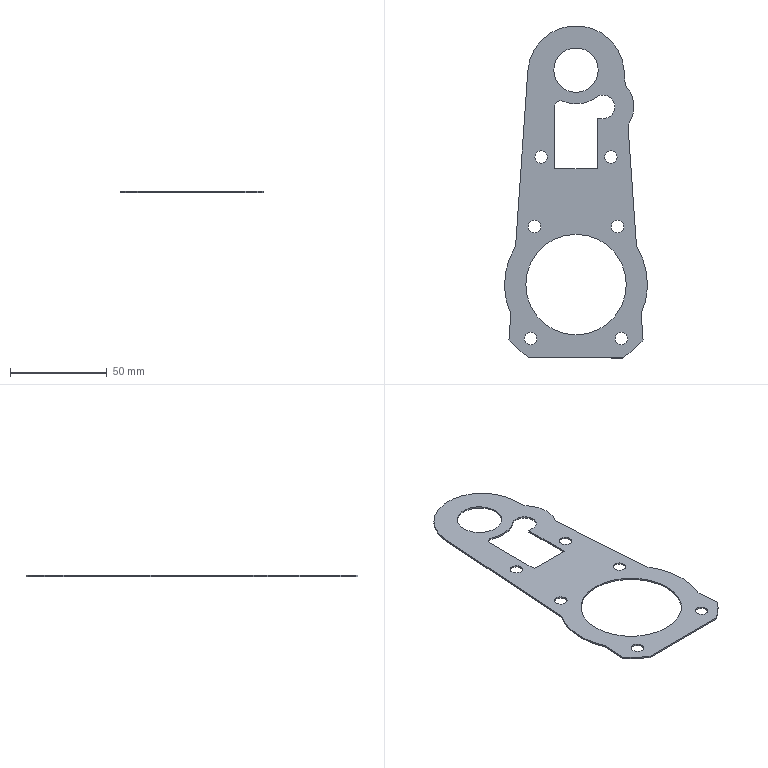Part | SolidWorks | features BaseBody 1 | 1 solid | 39 faces | box 74 x 172 x 0.8 mm | volume 5148 mm3 | cylinder 27 | plane 12 | commonest cylinder face diameters 6.5 x12 74 x3 12.2 x2 23 x2 52 x2 90 x2
STEP:
#1=CARTESIAN_POINT('',(-81.463,-50.104,-130.75));
#2=VERTEX_POINT('',#1);
#3=CARTESIAN_POINT('',(-78.207,-65.28,-130.75));
#4=VERTEX_POINT('',#3);
#5=CARTESIAN_POINT('',(-44.463,-50.104,-130.75));
#6=DIRECTION('',(0.,0.,1.));
#7=DIRECTION('',(1.,0.,0.));
#8=AXIS2_PLACEMENT_3D('',#5,#6,#7);
#9=CIRCLE('',#8,37.);
#10=EDGE_CURVE('',#2,#4,#9,.T.);
#11=ORIENTED_EDGE('',*,*,#10,.F.);
#12=CARTESIAN_POINT('',(-81.463,-50.104,-131.55));
#13=VERTEX_POINT('',#12);
#14=CARTESIAN_POINT('',(-81.463,-50.104,-130.75));
#15=DIRECTION('',(0.,0.,-1.));
#16=VECTOR('',#15,1000.);
#17=LINE('',#14,#16);
#18=EDGE_CURVE('',#2,#13,#17,.T.);
#19=ORIENTED_EDGE('',*,*,#18,.T.);
#20=CARTESIAN_POINT('',(-78.207,-65.28,-131.55));
#21=VERTEX_POINT('',#20);
#22=CARTESIAN_POINT('',(-44.463,-50.104,-131.55));
#23=DIRECTION('',(0.,0.,1.));
#24=DIRECTION('',(1.,0.,0.));
#25=AXIS2_PLACEMENT_3D('',#22,#23,#24);
#26=CIRCLE('',#25,37.);
#27=EDGE_CURVE('',#13,#21,#26,.T.);
#28=ORIENTED_EDGE('',*,*,#27,.T.);
#29=CARTESIAN_POINT('',(-78.207,-65.28,-130.75));
#30=DIRECTION('',(0.,0.,-1.));
#31=VECTOR('',#30,1000.);
#32=LINE('',#29,#31);
#33=EDGE_CURVE('',#4,#21,#32,.T.);
#34=ORIENTED_EDGE('',*,*,#33,.F.);
#35=EDGE_LOOP('',(#11,#19,#28,#34));
#36=FACE_OUTER_BOUND('',#35,.T.);
#37=CARTESIAN_POINT('',(-44.463,-50.104,-130.75));
#38=DIRECTION('',(0.,0.,-1.));
#39=DIRECTION('',(-1.,0.,0.));
#40=AXIS2_PLACEMENT_3D('',#37,#38,#39);
#41=CYLINDRICAL_SURFACE('',#40,37.);
#42=ADVANCED_FACE('',(#36),#41,.T.);
#43=CARTESIAN_POINT('',(-70.463,-50.104,-131.55));
#44=VERTEX_POINT('',#43);
#45=CARTESIAN_POINT('',(-18.463,-50.104,-131.55));
#46=VERTEX_POINT('',#45);
#47=CARTESIAN_POINT('',(-44.463,-50.104,-131.55));
#48=DIRECTION('',(0.,0.,1.));
#49=DIRECTION('',(1.,0.,0.));
#50=AXIS2_PLACEMENT_3D('',#47,#48,#49);
#51=CIRCLE('',#50,26.);
#52=EDGE_CURVE('',#44,#46,#51,.T.);
#53=ORIENTED_EDGE('',*,*,#52,.F.);
#54=CARTESIAN_POINT('',(-70.463,-50.104,-130.75));
#55=VERTEX_POINT('',#54);
#56=CARTESIAN_POINT('',(-70.463,-50.104,-131.55));
#57=DIRECTION('',(0.,0.,1.));
#58=VECTOR('',#57,1000.);
#59=LINE('',#56,#58);
#60=EDGE_CURVE('',#44,#55,#59,.T.);
#61=ORIENTED_EDGE('',*,*,#60,.T.);
#62=CARTESIAN_POINT('',(-18.463,-50.104,-130.75));
#63=VERTEX_POINT('',#62);
#64=CARTESIAN_POINT('',(-44.463,-50.104,-130.75));
#65=DIRECTION('',(0.,0.,1.));
#66=DIRECTION('',(1.,0.,0.));
#67=AXIS2_PLACEMENT_3D('',#64,#65,#66);
#68=CIRCLE('',#67,26.);
#69=EDGE_CURVE('',#55,#63,#68,.T.);
#70=ORIENTED_EDGE('',*,*,#69,.T.);
#71=CARTESIAN_POINT('',(-18.463,-50.104,-131.55));
#72=DIRECTION('',(0.,0.,1.));
#73=VECTOR('',#72,1000.);
#74=LINE('',#71,#73);
#75=EDGE_CURVE('',#46,#63,#74,.T.);
#76=ORIENTED_EDGE('',*,*,#75,.F.);
#77=EDGE_LOOP('',(#53,#61,#70,#76));
#78=FACE_OUTER_BOUND('',#77,.T.);
#79=CARTESIAN_POINT('',(-44.463,-50.104,-131.55));
#80=DIRECTION('',(0.,0.,1.));
#81=DIRECTION('',(1.,0.,0.));
#82=AXIS2_PLACEMENT_3D('',#79,#80,#81);
#83=CYLINDRICAL_SURFACE('',#82,26.);
#84=ADVANCED_FACE('',(#78),#83,.F.);
#85=CARTESIAN_POINT('',(-24.363,41.896,-131.55));
#86=VERTEX_POINT('',#85);
#87=CARTESIAN_POINT('',(-34.082,46.807,-131.55));
#88=VERTEX_POINT('',#87);
#89=CARTESIAN_POINT('',(-30.463,41.896,-131.55));
#90=DIRECTION('',(0.,0.,1.));
#91=DIRECTION('',(1.,0.,0.));
#92=AXIS2_PLACEMENT_3D('',#89,#90,#91);
#93=CIRCLE('',#92,6.1);
#94=EDGE_CURVE('',#86,#88,#93,.T.);
#95=ORIENTED_EDGE('',*,*,#94,.F.);
#96=CARTESIAN_POINT('',(-24.363,41.896,-130.75));
#97=VERTEX_POINT('',#96);
#98=CARTESIAN_POINT('',(-24.363,41.896,-131.55));
#99=DIRECTION('',(0.,0.,1.));
#100=VECTOR('',#99,1000.);
#101=LINE('',#98,#100);
#102=EDGE_CURVE('',#86,#97,#101,.T.);
#103=ORIENTED_EDGE('',*,*,#102,.T.);
#104=CARTESIAN_POINT('',(-34.082,46.807,-130.75));
#105=VERTEX_POINT('',#104);
#106=CARTESIAN_POINT('',(-30.463,41.896,-130.75));
#107=DIRECTION('',(0.,0.,1.));
#108=DIRECTION('',(1.,0.,0.));
#109=AXIS2_PLACEMENT_3D('',#106,#107,#108);
#110=CIRCLE('',#109,6.1);
#111=EDGE_CURVE('',#97,#105,#110,.T.);
#112=ORIENTED_EDGE('',*,*,#111,.T.);
#113=CARTESIAN_POINT('',(-34.082,46.807,-131.55));
#114=DIRECTION('',(0.,0.,1.));
#115=VECTOR('',#114,1000.);
#116=LINE('',#113,#115);
#117=EDGE_CURVE('',#88,#105,#116,.T.);
#118=ORIENTED_EDGE('',*,*,#117,.F.);
#119=EDGE_LOOP('',(#95,#103,#112,#118));
#120=FACE_OUTER_BOUND('',#119,.T.);
#121=CARTESIAN_POINT('',(-30.463,41.896,-131.55));
#122=DIRECTION('',(0.,0.,1.));
#123=DIRECTION('',(1.,0.,0.));
#124=AXIS2_PLACEMENT_3D('',#121,#122,#123);
#125=CYLINDRICAL_SURFACE('',#124,6.1);
#126=ADVANCED_FACE('',(#120),#125,.F.);
#127=CARTESIAN_POINT('',(-55.963,60.895,-131.55));
#128=VERTEX_POINT('',#127);
#129=CARTESIAN_POINT('',(-32.963,60.895,-131.55));
#130=VERTEX_POINT('',#129);
#131=CARTESIAN_POINT('',(-44.463,60.895,-131.55));
#132=DIRECTION('',(0.,0.,1.));
#133=DIRECTION('',(1.,0.,0.));
#134=AXIS2_PLACEMENT_3D('',#131,#132,#133);
#135=CIRCLE('',#134,11.5);
#136=EDGE_CURVE('',#128,#130,#135,.T.);
#137=ORIENTED_EDGE('',*,*,#136,.F.);
#138=CARTESIAN_POINT('',(-55.963,60.895,-130.75));
#139=VERTEX_POINT('',#138);
#140=CARTESIAN_POINT('',(-55.963,60.895,-131.55));
#141=DIRECTION('',(0.,0.,1.));
#142=VECTOR('',#141,1000.);
#143=LINE('',#140,#142);
#144=EDGE_CURVE('',#128,#139,#143,.T.);
#145=ORIENTED_EDGE('',*,*,#144,.T.);
#146=CARTESIAN_POINT('',(-32.963,60.895,-130.75));
#147=VERTEX_POINT('',#146);
#148=CARTESIAN_POINT('',(-44.463,60.895,-130.75));
#149=DIRECTION('',(0.,0.,1.));
#150=DIRECTION('',(1.,0.,0.));
#151=AXIS2_PLACEMENT_3D('',#148,#149,#150);
#152=CIRCLE('',#151,11.5);
#153=EDGE_CURVE('',#139,#147,#152,.T.);
#154=ORIENTED_EDGE('',*,*,#153,.T.);
#155=CARTESIAN_POINT('',(-32.963,60.895,-131.55));
#156=DIRECTION('',(0.,0.,1.));
#157=VECTOR('',#156,1000.);
#158=LINE('',#155,#157);
#159=EDGE_CURVE('',#130,#147,#158,.T.);
#160=ORIENTED_EDGE('',*,*,#159,.F.);
#161=EDGE_LOOP('',(#137,#145,#154,#160));
#162=FACE_OUTER_BOUND('',#161,.T.);
#163=CARTESIAN_POINT('',(-44.463,60.895,-131.55));
#164=DIRECTION('',(0.,0.,1.));
#165=DIRECTION('',(1.,0.,0.));
#166=AXIS2_PLACEMENT_3D('',#163,#164,#165);
#167=CYLINDRICAL_SURFACE('',#166,11.5);
#168=ADVANCED_FACE('',(#162),#167,.F.);
#169=CARTESIAN_POINT('',(-71.213,-78.104,-131.55));
#170=VERTEX_POINT('',#169);
#171=CARTESIAN_POINT('',(-64.713,-78.104,-131.55));
#172=VERTEX_POINT('',#171);
#173=CARTESIAN_POINT('',(-67.963,-78.104,-131.55));
#174=DIRECTION('',(0.,0.,1.));
#175=DIRECTION('',(1.,0.,0.));
#176=AXIS2_PLACEMENT_3D('',#173,#174,#175);
#177=CIRCLE('',#176,3.25);
#178=EDGE_CURVE('',#170,#172,#177,.T.);
#179=ORIENTED_EDGE('',*,*,#178,.F.);
#180=CARTESIAN_POINT('',(-71.213,-78.104,-130.75));
#181=VERTEX_POINT('',#180);
#182=CARTESIAN_POINT('',(-71.213,-78.104,-131.55));
#183=DIRECTION('',(0.,0.,1.));
#184=VECTOR('',#183,1000.);
#185=LINE('',#182,#184);
#186=EDGE_CURVE('',#170,#181,#185,.T.);
#187=ORIENTED_EDGE('',*,*,#186,.T.);
#188=CARTESIAN_POINT('',(-64.713,-78.104,-130.75));
#189=VERTEX_POINT('',#188);
#190=CARTESIAN_POINT('',(-67.963,-78.104,-130.75));
#191=DIRECTION('',(0.,0.,1.));
#192=DIRECTION('',(1.,0.,0.));
#193=AXIS2_PLACEMENT_3D('',#190,#191,#192);
#194=CIRCLE('',#193,3.25);
#195=EDGE_CURVE('',#181,#189,#194,.T.);
#196=ORIENTED_EDGE('',*,*,#195,.T.);
#197=CARTESIAN_POINT('',(-64.713,-78.104,-131.55));
#198=DIRECTION('',(0.,0.,1.));
#199=VECTOR('',#198,1000.);
#200=LINE('',#197,#199);
#201=EDGE_CURVE('',#172,#189,#200,.T.);
#202=ORIENTED_EDGE('',*,*,#201,.F.);
#203=EDGE_LOOP('',(#179,#187,#196,#202));
#204=FACE_OUTER_BOUND('',#203,.T.);
#205=CARTESIAN_POINT('',(-67.963,-78.104,-131.55));
#206=DIRECTION('',(0.,0.,1.));
#207=DIRECTION('',(1.,0.,0.));
#208=AXIS2_PLACEMENT_3D('',#205,#206,#207);
#209=CYLINDRICAL_SURFACE('',#208,3.25);
#210=ADVANCED_FACE('',(#204),#209,.F.);
#211=CARTESIAN_POINT('',(-17.713,-78.104,-131.55));
#212=VERTEX_POINT('',#211);
#213=CARTESIAN_POINT('',(-24.213,-78.104,-131.55));
#214=VERTEX_POINT('',#213);
#215=CARTESIAN_POINT('',(-20.963,-78.104,-131.55));
#216=DIRECTION('',(0.,0.,-1.));
#217=DIRECTION('',(-1.,0.,0.));
#218=AXIS2_PLACEMENT_3D('',#215,#216,#217);
#219=CIRCLE('',#218,3.25);
#220=EDGE_CURVE('',#212,#214,#219,.T.);
#221=ORIENTED_EDGE('',*,*,#220,.T.);
#222=CARTESIAN_POINT('',(-24.213,-78.104,-130.75));
#223=VERTEX_POINT('',#222);
#224=CARTESIAN_POINT('',(-24.213,-78.104,-131.55));
#225=DIRECTION('',(0.,0.,1.));
#226=VECTOR('',#225,1000.);
#227=LINE('',#224,#226);
#228=EDGE_CURVE('',#214,#223,#227,.T.);
#229=ORIENTED_EDGE('',*,*,#228,.T.);
#230=CARTESIAN_POINT('',(-17.713,-78.104,-130.75));
#231=VERTEX_POINT('',#230);
#232=CARTESIAN_POINT('',(-20.963,-78.104,-130.75));
#233=DIRECTION('',(0.,0.,-1.));
#234=DIRECTION('',(-1.,0.,0.));
#235=AXIS2_PLACEMENT_3D('',#232,#233,#234);
#236=CIRCLE('',#235,3.25);
#237=EDGE_CURVE('',#231,#223,#236,.T.);
#238=ORIENTED_EDGE('',*,*,#237,.F.);
#239=CARTESIAN_POINT('',(-17.713,-78.104,-131.55));
#240=DIRECTION('',(0.,0.,1.));
#241=VECTOR('',#240,1000.);
#242=LINE('',#239,#241);
#243=EDGE_CURVE('',#212,#231,#242,.T.);
#244=ORIENTED_EDGE('',*,*,#243,.F.);
#245=EDGE_LOOP('',(#221,#229,#238,#244));
#246=FACE_OUTER_BOUND('',#245,.T.);
#247=CARTESIAN_POINT('',(-20.963,-78.104,-131.55));
#248=DIRECTION('',(0.,0.,1.));
#249=DIRECTION('',(1.,0.,0.));
#250=AXIS2_PLACEMENT_3D('',#247,#248,#249);
#251=CYLINDRICAL_SURFACE('',#250,3.25);
#252=ADVANCED_FACE('',(#246),#251,.F.);
#253=CARTESIAN_POINT('',(-69.213,-20.104,-131.55));
#254=VERTEX_POINT('',#253);
#255=CARTESIAN_POINT('',(-62.713,-20.104,-131.55));
#256=VERTEX_POINT('',#255);
#257=CARTESIAN_POINT('',(-65.963,-20.104,-131.55));
#258=DIRECTION('',(0.,0.,1.));
#259=DIRECTION('',(1.,0.,0.));
#260=AXIS2_PLACEMENT_3D('',#257,#258,#259);
#261=CIRCLE('',#260,3.25);
#262=EDGE_CURVE('',#254,#256,#261,.T.);
#263=ORIENTED_EDGE('',*,*,#262,.F.);
#264=CARTESIAN_POINT('',(-69.213,-20.104,-130.75));
#265=VERTEX_POINT('',#264);
#266=CARTESIAN_POINT('',(-69.213,-20.104,-131.55));
#267=DIRECTION('',(0.,0.,1.));
#268=VECTOR('',#267,1000.);
#269=LINE('',#266,#268);
#270=EDGE_CURVE('',#254,#265,#269,.T.);
#271=ORIENTED_EDGE('',*,*,#270,.T.);
#272=CARTESIAN_POINT('',(-62.713,-20.104,-130.75));
#273=VERTEX_POINT('',#272);
#274=CARTESIAN_POINT('',(-65.963,-20.104,-130.75));
#275=DIRECTION('',(0.,0.,1.));
#276=DIRECTION('',(1.,0.,0.));
#277=AXIS2_PLACEMENT_3D('',#274,#275,#276);
#278=CIRCLE('',#277,3.25);
#279=EDGE_CURVE('',#265,#273,#278,.T.);
#280=ORIENTED_EDGE('',*,*,#279,.T.);
#281=CARTESIAN_POINT('',(-62.713,-20.104,-131.55));
#282=DIRECTION('',(0.,0.,1.));
#283=VECTOR('',#282,1000.);
#284=LINE('',#281,#283);
#285=EDGE_CURVE('',#256,#273,#284,.T.);
#286=ORIENTED_EDGE('',*,*,#285,.F.);
#287=EDGE_LOOP('',(#263,#271,#280,#286));
#288=FACE_OUTER_BOUND('',#287,.T.);
#289=CARTESIAN_POINT('',(-65.963,-20.104,-131.55));
#290=DIRECTION('',(0.,0.,1.));
#291=DIRECTION('',(1.,0.,0.));
#292=AXIS2_PLACEMENT_3D('',#289,#290,#291);
#293=CYLINDRICAL_SURFACE('',#292,3.25);
#294=ADVANCED_FACE('',(#288),#293,.F.);
#295=CARTESIAN_POINT('',(-19.713,-20.104,-131.55));
#296=VERTEX_POINT('',#295);
#297=CARTESIAN_POINT('',(-26.213,-20.104,-131.55));
#298=VERTEX_POINT('',#297);
#299=CARTESIAN_POINT('',(-22.963,-20.104,-131.55));
#300=DIRECTION('',(0.,0.,-1.));
#301=DIRECTION('',(-1.,0.,0.));
#302=AXIS2_PLACEMENT_3D('',#299,#300,#301);
#303=CIRCLE('',#302,3.25);
#304=EDGE_CURVE('',#296,#298,#303,.T.);
#305=ORIENTED_EDGE('',*,*,#304,.T.);
#306=CARTESIAN_POINT('',(-26.213,-20.104,-130.75));
#307=VERTEX_POINT('',#306);
#308=CARTESIAN_POINT('',(-26.213,-20.104,-131.55));
#309=DIRECTION('',(0.,0.,1.));
#310=VECTOR('',#309,1000.);
#311=LINE('',#308,#310);
#312=EDGE_CURVE('',#298,#307,#311,.T.);
#313=ORIENTED_EDGE('',*,*,#312,.T.);
#314=CARTESIAN_POINT('',(-19.713,-20.104,-130.75));
#315=VERTEX_POINT('',#314);
#316=CARTESIAN_POINT('',(-22.963,-20.104,-130.75));
#317=DIRECTION('',(0.,0.,-1.));
#318=DIRECTION('',(-1.,0.,0.));
#319=AXIS2_PLACEMENT_3D('',#316,#317,#318);
#320=CIRCLE('',#319,3.25);
#321=EDGE_CURVE('',#315,#307,#320,.T.);
#322=ORIENTED_EDGE('',*,*,#321,.F.);
#323=CARTESIAN_POINT('',(-19.713,-20.104,-131.55));
#324=DIRECTION('',(0.,0.,1.));
#325=VECTOR('',#324,1000.);
#326=LINE('',#323,#325);
#327=EDGE_CURVE('',#296,#315,#326,.T.);
#328=ORIENTED_EDGE('',*,*,#327,.F.);
#329=EDGE_LOOP('',(#305,#313,#322,#328));
#330=FACE_OUTER_BOUND('',#329,.T.);
#331=CARTESIAN_POINT('',(-22.963,-20.104,-131.55));
#332=DIRECTION('',(0.,0.,1.));
#333=DIRECTION('',(1.,0.,0.));
#334=AXIS2_PLACEMENT_3D('',#331,#332,#333);
#335=CYLINDRICAL_SURFACE('',#334,3.25);
#336=ADVANCED_FACE('',(#330),#335,.F.);
#337=CARTESIAN_POINT('',(-65.713,15.896,-131.55));
#338=VERTEX_POINT('',#337);
#339=CARTESIAN_POINT('',(-59.213,15.896,-131.55));
#340=VERTEX_POINT('',#339);
#341=CARTESIAN_POINT('',(-62.463,15.896,-131.55));
#342=DIRECTION('',(0.,0.,1.));
#343=DIRECTION('',(1.,0.,0.));
#344=AXIS2_PLACEMENT_3D('',#341,#342,#343);
#345=CIRCLE('',#344,3.25);
#346=EDGE_CURVE('',#338,#340,#345,.T.);
#347=ORIENTED_EDGE('',*,*,#346,.F.);
#348=CARTESIAN_POINT('',(-65.713,15.896,-130.75));
#349=VERTEX_POINT('',#348);
#350=CARTESIAN_POINT('',(-65.713,15.896,-131.55));
#351=DIRECTION('',(0.,0.,1.));
#352=VECTOR('',#351,1000.);
#353=LINE('',#350,#352);
#354=EDGE_CURVE('',#338,#349,#353,.T.);
#355=ORIENTED_EDGE('',*,*,#354,.T.);
#356=CARTESIAN_POINT('',(-59.213,15.896,-130.75));
#357=VERTEX_POINT('',#356);
#358=CARTESIAN_POINT('',(-62.463,15.896,-130.75));
#359=DIRECTION('',(0.,0.,1.));
#360=DIRECTION('',(1.,0.,0.));
#361=AXIS2_PLACEMENT_3D('',#358,#359,#360);
#362=CIRCLE('',#361,3.25);
#363=EDGE_CURVE('',#349,#357,#362,.T.);
#364=ORIENTED_EDGE('',*,*,#363,.T.);
#365=CARTESIAN_POINT('',(-59.213,15.896,-131.55));
#366=DIRECTION('',(0.,0.,1.));
#367=VECTOR('',#366,1000.);
#368=LINE('',#365,#367);
#369=EDGE_CURVE('',#340,#357,#368,.T.);
#370=ORIENTED_EDGE('',*,*,#369,.F.);
#371=EDGE_LOOP('',(#347,#355,#364,#370));
#372=FACE_OUTER_BOUND('',#371,.T.);
#373=CARTESIAN_POINT('',(-62.463,15.896,-131.55));
#374=DIRECTION('',(0.,0.,1.));
#375=DIRECTION('',(1.,0.,0.));
#376=AXIS2_PLACEMENT_3D('',#373,#374,#375);
#377=CYLINDRICAL_SURFACE('',#376,3.25);
#378=ADVANCED_FACE('',(#372),#377,.F.);
#379=CARTESIAN_POINT('',(-23.213,15.896,-131.55));
#380=VERTEX_POINT('',#379);
#381=CARTESIAN_POINT('',(-29.713,15.896,-131.55));
#382=VERTEX_POINT('',#381);
#383=CARTESIAN_POINT('',(-26.463,15.896,-131.55));
#384=DIRECTION('',(0.,0.,-1.));
#385=DIRECTION('',(-1.,0.,0.));
#386=AXIS2_PLACEMENT_3D('',#383,#384,#385);
#387=CIRCLE('',#386,3.25);
#388=EDGE_CURVE('',#380,#382,#387,.T.);
#389=ORIENTED_EDGE('',*,*,#388,.T.);
#390=CARTESIAN_POINT('',(-29.713,15.896,-130.75));
#391=VERTEX_POINT('',#390);
#392=CARTESIAN_POINT('',(-29.713,15.896,-131.55));
#393=DIRECTION('',(0.,0.,1.));
#394=VECTOR('',#393,1000.);
#395=LINE('',#392,#394);
#396=EDGE_CURVE('',#382,#391,#395,.T.);
#397=ORIENTED_EDGE('',*,*,#396,.T.);
#398=CARTESIAN_POINT('',(-23.213,15.896,-130.75));
#399=VERTEX_POINT('',#398);
#400=CARTESIAN_POINT('',(-26.463,15.896,-130.75));
#401=DIRECTION('',(0.,0.,-1.));
#402=DIRECTION('',(-1.,0.,0.));
#403=AXIS2_PLACEMENT_3D('',#400,#401,#402);
#404=CIRCLE('',#403,3.25);
#405=EDGE_CURVE('',#399,#391,#404,.T.);
#406=ORIENTED_EDGE('',*,*,#405,.F.);
#407=CARTESIAN_POINT('',(-23.213,15.896,-131.55));
#408=DIRECTION('',(0.,0.,1.));
#409=VECTOR('',#408,1000.);
#410=LINE('',#407,#409);
#411=EDGE_CURVE('',#380,#399,#410,.T.);
#412=ORIENTED_EDGE('',*,*,#411,.F.);
#413=EDGE_LOOP('',(#389,#397,#406,#412));
#414=FACE_OUTER_BOUND('',#413,.T.);
#415=CARTESIAN_POINT('',(-26.463,15.896,-131.55));
#416=DIRECTION('',(0.,0.,1.));
#417=DIRECTION('',(1.,0.,0.));
#418=AXIS2_PLACEMENT_3D('',#415,#416,#417);
#419=CYLINDRICAL_SURFACE('',#418,3.25);
#420=ADVANCED_FACE('',(#414),#419,.F.);
#421=ORIENTED_EDGE('',*,*,#396,.F.);
#422=CARTESIAN_POINT('',(-26.463,15.896,-131.55));
#423=DIRECTION('',(0.,0.,-1.));
#424=DIRECTION('',(-1.,0.,0.));
#425=AXIS2_PLACEMENT_3D('',#422,#423,#424);
#426=CIRCLE('',#425,3.25);
#427=EDGE_CURVE('',#382,#380,#426,.T.);
#428=ORIENTED_EDGE('',*,*,#427,.T.);
#429=ORIENTED_EDGE('',*,*,#411,.T.);
#430=CARTESIAN_POINT('',(-26.463,15.896,-130.75));
#431=DIRECTION('',(0.,0.,-1.));
#432=DIRECTION('',(-1.,0.,0.));
#433=AXIS2_PLACEMENT_3D('',#430,#431,#432);
#434=CIRCLE('',#433,3.25);
#435=EDGE_CURVE('',#391,#399,#434,.T.);
#436=ORIENTED_EDGE('',*,*,#435,.F.);
#437=EDGE_LOOP('',(#421,#428,#429,#436));
#438=FACE_OUTER_BOUND('',#437,.T.);
#439=CARTESIAN_POINT('',(-26.463,15.896,-131.55));
#440=DIRECTION('',(0.,0.,1.));
#441=DIRECTION('',(1.,0.,0.));
#442=AXIS2_PLACEMENT_3D('',#439,#440,#441);
#443=CYLINDRICAL_SURFACE('',#442,3.25);
#444=ADVANCED_FACE('',(#438),#443,.F.);
#445=ORIENTED_EDGE('',*,*,#354,.F.);
#446=CARTESIAN_POINT('',(-62.463,15.896,-131.55));
#447=DIRECTION('',(0.,0.,1.));
#448=DIRECTION('',(1.,0.,0.));
#449=AXIS2_PLACEMENT_3D('',#446,#447,#448);
#450=CIRCLE('',#449,3.25);
#451=EDGE_CURVE('',#340,#338,#450,.T.);
#452=ORIENTED_EDGE('',*,*,#451,.F.);
#453=ORIENTED_EDGE('',*,*,#369,.T.);
#454=CARTESIAN_POINT('',(-62.463,15.896,-130.75));
#455=DIRECTION('',(0.,0.,1.));
#456=DIRECTION('',(1.,0.,0.));
#457=AXIS2_PLACEMENT_3D('',#454,#455,#456);
#458=CIRCLE('',#457,3.25);
#459=EDGE_CURVE('',#357,#349,#458,.T.);
#460=ORIENTED_EDGE('',*,*,#459,.T.);
#461=EDGE_LOOP('',(#445,#452,#453,#460));
#462=FACE_OUTER_BOUND('',#461,.T.);
#463=CARTESIAN_POINT('',(-62.463,15.896,-131.55));
#464=DIRECTION('',(0.,0.,1.));
#465=DIRECTION('',(1.,0.,0.));
#466=AXIS2_PLACEMENT_3D('',#463,#464,#465);
#467=CYLINDRICAL_SURFACE('',#466,3.25);
#468=ADVANCED_FACE('',(#462),#467,.F.);
#469=ORIENTED_EDGE('',*,*,#312,.F.);
#470=CARTESIAN_POINT('',(-22.963,-20.104,-131.55));
#471=DIRECTION('',(0.,0.,-1.));
#472=DIRECTION('',(-1.,0.,0.));
#473=AXIS2_PLACEMENT_3D('',#470,#471,#472);
#474=CIRCLE('',#473,3.25);
#475=EDGE_CURVE('',#298,#296,#474,.T.);
#476=ORIENTED_EDGE('',*,*,#475,.T.);
#477=ORIENTED_EDGE('',*,*,#327,.T.);
#478=CARTESIAN_POINT('',(-22.963,-20.104,-130.75));
#479=DIRECTION('',(0.,0.,-1.));
#480=DIRECTION('',(-1.,0.,0.));
#481=AXIS2_PLACEMENT_3D('',#478,#479,#480);
#482=CIRCLE('',#481,3.25);
#483=EDGE_CURVE('',#307,#315,#482,.T.);
#484=ORIENTED_EDGE('',*,*,#483,.F.);
#485=EDGE_LOOP('',(#469,#476,#477,#484));
#486=FACE_OUTER_BOUND('',#485,.T.);
#487=CARTESIAN_POINT('',(-22.963,-20.104,-131.55));
#488=DIRECTION('',(0.,0.,1.));
#489=DIRECTION('',(1.,0.,0.));
#490=AXIS2_PLACEMENT_3D('',#487,#488,#489);
#491=CYLINDRICAL_SURFACE('',#490,3.25);
#492=ADVANCED_FACE('',(#486),#491,.F.);
#493=ORIENTED_EDGE('',*,*,#270,.F.);
#494=CARTESIAN_POINT('',(-65.963,-20.104,-131.55));
#495=DIRECTION('',(0.,0.,1.));
#496=DIRECTION('',(1.,0.,0.));
#497=AXIS2_PLACEMENT_3D('',#494,#495,#496);
#498=CIRCLE('',#497,3.25);
#499=EDGE_CURVE('',#256,#254,#498,.T.);
#500=ORIENTED_EDGE('',*,*,#499,.F.);
#501=ORIENTED_EDGE('',*,*,#285,.T.);
#502=CARTESIAN_POINT('',(-65.963,-20.104,-130.75));
#503=DIRECTION('',(0.,0.,1.));
#504=DIRECTION('',(1.,0.,0.));
#505=AXIS2_PLACEMENT_3D('',#502,#503,#504);
#506=CIRCLE('',#505,3.25);
#507=EDGE_CURVE('',#273,#265,#506,.T.);
#508=ORIENTED_EDGE('',*,*,#507,.T.);
#509=EDGE_LOOP('',(#493,#500,#501,#508));
#510=FACE_OUTER_BOUND('',#509,.T.);
#511=CARTESIAN_POINT('',(-65.963,-20.104,-131.55));
#512=DIRECTION('',(0.,0.,1.));
#513=DIRECTION('',(1.,0.,0.));
#514=AXIS2_PLACEMENT_3D('',#511,#512,#513);
#515=CYLINDRICAL_SURFACE('',#514,3.25);
#516=ADVANCED_FACE('',(#510),#515,.F.);
#517=ORIENTED_EDGE('',*,*,#228,.F.);
#518=CARTESIAN_POINT('',(-20.963,-78.104,-131.55));
#519=DIRECTION('',(0.,0.,-1.));
#520=DIRECTION('',(-1.,0.,0.));
#521=AXIS2_PLACEMENT_3D('',#518,#519,#520);
#522=CIRCLE('',#521,3.25);
#523=EDGE_CURVE('',#214,#212,#522,.T.);
#524=ORIENTED_EDGE('',*,*,#523,.T.);
#525=ORIENTED_EDGE('',*,*,#243,.T.);
#526=CARTESIAN_POINT('',(-20.963,-78.104,-130.75));
#527=DIRECTION('',(0.,0.,-1.));
#528=DIRECTION('',(-1.,0.,0.));
#529=AXIS2_PLACEMENT_3D('',#526,#527,#528);
#530=CIRCLE('',#529,3.25);
#531=EDGE_CURVE('',#223,#231,#530,.T.);
#532=ORIENTED_EDGE('',*,*,#531,.F.);
#533=EDGE_LOOP('',(#517,#524,#525,#532));
#534=FACE_OUTER_BOUND('',#533,.T.);
#535=CARTESIAN_POINT('',(-20.963,-78.104,-131.55));
#536=DIRECTION('',(0.,0.,1.));
#537=DIRECTION('',(1.,0.,0.));
#538=AXIS2_PLACEMENT_3D('',#535,#536,#537);
#539=CYLINDRICAL_SURFACE('',#538,3.25);
#540=ADVANCED_FACE('',(#534),#539,.F.);
#541=ORIENTED_EDGE('',*,*,#186,.F.);
#542=CARTESIAN_POINT('',(-67.963,-78.104,-131.55));
#543=DIRECTION('',(0.,0.,1.));
#544=DIRECTION('',(1.,0.,0.));
#545=AXIS2_PLACEMENT_3D('',#542,#543,#544);
#546=CIRCLE('',#545,3.25);
#547=EDGE_CURVE('',#172,#170,#546,.T.);
#548=ORIENTED_EDGE('',*,*,#547,.F.);
#549=ORIENTED_EDGE('',*,*,#201,.T.);
#550=CARTESIAN_POINT('',(-67.963,-78.104,-130.75));
#551=DIRECTION('',(0.,0.,1.));
#552=DIRECTION('',(1.,0.,0.));
#553=AXIS2_PLACEMENT_3D('',#550,#551,#552);
#554=CIRCLE('',#553,3.25);
#555=EDGE_CURVE('',#189,#181,#554,.T.);
#556=ORIENTED_EDGE('',*,*,#555,.T.);
#557=EDGE_LOOP('',(#541,#548,#549,#556));
#558=FACE_OUTER_BOUND('',#557,.T.);
#559=CARTESIAN_POINT('',(-67.963,-78.104,-131.55));
#560=DIRECTION('',(0.,0.,1.));
#561=DIRECTION('',(1.,0.,0.));
#562=AXIS2_PLACEMENT_3D('',#559,#560,#561);
#563=CYLINDRICAL_SURFACE('',#562,3.25);
#564=ADVANCED_FACE('',(#558),#563,.F.);
#565=ORIENTED_EDGE('',*,*,#144,.F.);
#566=CARTESIAN_POINT('',(-44.463,60.895,-131.55));
#567=DIRECTION('',(0.,0.,1.));
#568=DIRECTION('',(1.,0.,0.));
#569=AXIS2_PLACEMENT_3D('',#566,#567,#568);
#570=CIRCLE('',#569,11.5);
#571=EDGE_CURVE('',#130,#128,#570,.T.);
#572=ORIENTED_EDGE('',*,*,#571,.F.);
#573=ORIENTED_EDGE('',*,*,#159,.T.);
#574=CARTESIAN_POINT('',(-44.463,60.895,-130.75));
#575=DIRECTION('',(0.,0.,1.));
#576=DIRECTION('',(1.,0.,0.));
#577=AXIS2_PLACEMENT_3D('',#574,#575,#576);
#578=CIRCLE('',#577,11.5);
#579=EDGE_CURVE('',#147,#139,#578,.T.);
#580=ORIENTED_EDGE('',*,*,#579,.T.);
#581=EDGE_LOOP('',(#565,#572,#573,#580));
#582=FACE_OUTER_BOUND('',#581,.T.);
#583=CARTESIAN_POINT('',(-44.463,60.895,-131.55));
#584=DIRECTION('',(0.,0.,1.));
#585=DIRECTION('',(1.,0.,0.));
#586=AXIS2_PLACEMENT_3D('',#583,#584,#585);
#587=CYLINDRICAL_SURFACE('',#586,11.5);
#588=ADVANCED_FACE('',(#582),#587,.F.);
#589=ORIENTED_EDGE('',*,*,#102,.F.);
#590=CARTESIAN_POINT('',(-30.463,35.796,-131.55));
#591=VERTEX_POINT('',#590);
#592=CARTESIAN_POINT('',(-30.463,41.896,-131.55));
#593=DIRECTION('',(0.,0.,1.));
#594=DIRECTION('',(1.,0.,0.));
#595=AXIS2_PLACEMENT_3D('',#592,#593,#594);
#596=CIRCLE('',#595,6.1);
#597=EDGE_CURVE('',#591,#86,#596,.T.);
#598=ORIENTED_EDGE('',*,*,#597,.F.);
#599=CARTESIAN_POINT('',(-30.463,35.796,-130.75));
#600=VERTEX_POINT('',#599);
#601=CARTESIAN_POINT('',(-30.463,35.796,-131.55));
#602=DIRECTION('',(0.,0.,1.));
#603=VECTOR('',#602,1000.);
#604=LINE('',#601,#603);
#605=EDGE_CURVE('',#591,#600,#604,.T.);
#606=ORIENTED_EDGE('',*,*,#605,.T.);
#607=CARTESIAN_POINT('',(-30.463,41.896,-130.75));
#608=DIRECTION('',(0.,0.,1.));
#609=DIRECTION('',(1.,0.,0.));
#610=AXIS2_PLACEMENT_3D('',#607,#608,#609);
#611=CIRCLE('',#610,6.1);
#612=EDGE_CURVE('',#600,#97,#611,.T.);
#613=ORIENTED_EDGE('',*,*,#612,.T.);
#614=EDGE_LOOP('',(#589,#598,#606,#613));
#615=FACE_OUTER_BOUND('',#614,.T.);
#616=CARTESIAN_POINT('',(-30.463,41.896,-131.55));
#617=DIRECTION('',(0.,0.,1.));
#618=DIRECTION('',(1.,0.,0.));
#619=AXIS2_PLACEMENT_3D('',#616,#617,#618);
#620=CYLINDRICAL_SURFACE('',#619,6.1);
#621=ADVANCED_FACE('',(#615),#620,.F.);
#622=ORIENTED_EDGE('',*,*,#117,.T.);
#623=CARTESIAN_POINT('',(-51.321,44.795,-130.75));
#624=VERTEX_POINT('',#623);
#625=CARTESIAN_POINT('',(-44.463,60.895,-130.75));
#626=DIRECTION('',(0.,0.,1.));
#627=DIRECTION('',(1.,0.,0.));
#628=AXIS2_PLACEMENT_3D('',#625,#626,#627);
#629=CIRCLE('',#628,17.5);
#630=EDGE_CURVE('',#624,#105,#629,.T.);
#631=ORIENTED_EDGE('',*,*,#630,.F.);
#632=CARTESIAN_POINT('',(-51.321,44.795,-131.55));
#633=VERTEX_POINT('',#632);
#634=CARTESIAN_POINT('',(-51.321,44.795,-131.55));
#635=DIRECTION('',(0.,0.,1.));
#636=VECTOR('',#635,1000.);
#637=LINE('',#634,#636);
#638=EDGE_CURVE('',#633,#624,#637,.T.);
#639=ORIENTED_EDGE('',*,*,#638,.F.);
#640=CARTESIAN_POINT('',(-44.463,60.895,-131.55));
#641=DIRECTION('',(0.,0.,1.));
#642=DIRECTION('',(1.,0.,0.));
#643=AXIS2_PLACEMENT_3D('',#640,#641,#642);
#644=CIRCLE('',#643,17.5);
#645=EDGE_CURVE('',#633,#88,#644,.T.);
#646=ORIENTED_EDGE('',*,*,#645,.T.);
#647=EDGE_LOOP('',(#622,#631,#639,#646));
#648=FACE_OUTER_BOUND('',#647,.T.);
#649=CARTESIAN_POINT('',(-44.463,60.895,-131.55));
#650=DIRECTION('',(0.,0.,1.));
#651=DIRECTION('',(1.,0.,0.));
#652=AXIS2_PLACEMENT_3D('',#649,#650,#651);
#653=CYLINDRICAL_SURFACE('',#652,17.5);
#654=ADVANCED_FACE('',(#648),#653,.T.);
#655=ORIENTED_EDGE('',*,*,#638,.T.);
#656=CARTESIAN_POINT('',(-55.497,42.035,-130.75));
#657=VERTEX_POINT('',#656);
#658=CARTESIAN_POINT('',(-52.497,42.035,-130.75));
#659=DIRECTION('',(0.,0.,-1.));
#660=DIRECTION('',(-1.,0.,0.));
#661=AXIS2_PLACEMENT_3D('',#658,#659,#660);
#662=CIRCLE('',#661,3.);
#663=EDGE_CURVE('',#657,#624,#662,.T.);
#664=ORIENTED_EDGE('',*,*,#663,.F.);
#665=CARTESIAN_POINT('',(-55.497,42.035,-131.55));
#666=VERTEX_POINT('',#665);
#667=CARTESIAN_POINT('',(-55.497,42.035,-131.55));
#668=DIRECTION('',(0.,0.,1.));
#669=VECTOR('',#668,1000.);
#670=LINE('',#667,#669);
#671=EDGE_CURVE('',#666,#657,#670,.T.);
#672=ORIENTED_EDGE('',*,*,#671,.F.);
#673=CARTESIAN_POINT('',(-52.497,42.035,-131.55));
#674=DIRECTION('',(0.,0.,-1.));
#675=DIRECTION('',(-1.,0.,0.));
#676=AXIS2_PLACEMENT_3D('',#673,#674,#675);
#677=CIRCLE('',#676,3.);
#678=EDGE_CURVE('',#666,#633,#677,.T.);
#679=ORIENTED_EDGE('',*,*,#678,.T.);
#680=EDGE_LOOP('',(#655,#664,#672,#679));
#681=FACE_OUTER_BOUND('',#680,.T.);
#682=CARTESIAN_POINT('',(-52.497,42.035,-131.55));
#683=DIRECTION('',(0.,0.,1.));
#684=DIRECTION('',(1.,0.,0.));
#685=AXIS2_PLACEMENT_3D('',#682,#683,#684);
#686=CYLINDRICAL_SURFACE('',#685,3.);
#687=ADVANCED_FACE('',(#681),#686,.F.);
#688=ORIENTED_EDGE('',*,*,#671,.T.);
#689=CARTESIAN_POINT('',(-55.497,9.896,-130.75));
#690=VERTEX_POINT('',#689);
#691=CARTESIAN_POINT('',(-55.497,42.035,-130.75));
#692=DIRECTION('',(0.,-1.,0.));
#693=VECTOR('',#692,1000.);
#694=LINE('',#691,#693);
#695=EDGE_CURVE('',#657,#690,#694,.T.);
#696=ORIENTED_EDGE('',*,*,#695,.T.);
#697=CARTESIAN_POINT('',(-55.497,9.896,-131.55));
#698=VERTEX_POINT('',#697);
#699=CARTESIAN_POINT('',(-55.497,9.896,-131.55));
#700=DIRECTION('',(0.,0.,1.));
#701=VECTOR('',#700,1000.);
#702=LINE('',#699,#701);
#703=EDGE_CURVE('',#698,#690,#702,.T.);
#704=ORIENTED_EDGE('',*,*,#703,.F.);
#705=CARTESIAN_POINT('',(-55.497,42.035,-131.55));
#706=DIRECTION('',(0.,-1.,0.));
#707=VECTOR('',#706,1000.);
#708=LINE('',#705,#707);
#709=EDGE_CURVE('',#666,#698,#708,.T.);
#710=ORIENTED_EDGE('',*,*,#709,.F.);
#711=EDGE_LOOP('',(#688,#696,#704,#710));
#712=FACE_OUTER_BOUND('',#711,.T.);
#713=CARTESIAN_POINT('',(-55.497,42.035,-131.55));
#714=DIRECTION('',(-1.,0.,0.));
#715=DIRECTION('',(0.,0.,1.));
#716=AXIS2_PLACEMENT_3D('',#713,#714,#715);
#717=PLANE('',#716);
#718=ADVANCED_FACE('',(#712),#717,.F.);
#719=ORIENTED_EDGE('',*,*,#703,.T.);
#720=CARTESIAN_POINT('',(-33.429,9.896,-130.75));
#721=VERTEX_POINT('',#720);
#722=CARTESIAN_POINT('',(-33.429,9.896,-130.75));
#723=DIRECTION('',(-1.,0.,0.));
#724=VECTOR('',#723,1000.);
#725=LINE('',#722,#724);
#726=EDGE_CURVE('',#721,#690,#725,.T.);
#727=ORIENTED_EDGE('',*,*,#726,.F.);
#728=CARTESIAN_POINT('',(-33.429,9.896,-131.55));
#729=VERTEX_POINT('',#728);
#730=CARTESIAN_POINT('',(-33.429,9.896,-131.55));
#731=DIRECTION('',(0.,0.,1.));
#732=VECTOR('',#731,1000.);
#733=LINE('',#730,#732);
#734=EDGE_CURVE('',#729,#721,#733,.T.);
#735=ORIENTED_EDGE('',*,*,#734,.F.);
#736=CARTESIAN_POINT('',(-33.429,9.896,-131.55));
#737=DIRECTION('',(-1.,0.,0.));
#738=VECTOR('',#737,1000.);
#739=LINE('',#736,#738);
#740=EDGE_CURVE('',#729,#698,#739,.T.);
#741=ORIENTED_EDGE('',*,*,#740,.T.);
#742=EDGE_LOOP('',(#719,#727,#735,#741));
#743=FACE_OUTER_BOUND('',#742,.T.);
#744=CARTESIAN_POINT('',(-33.429,9.896,-131.55));
#745=DIRECTION('',(0.,1.,0.));
#746=DIRECTION('',(1.,0.,0.));
#747=AXIS2_PLACEMENT_3D('',#744,#745,#746);
#748=PLANE('',#747);
#749=ADVANCED_FACE('',(#743),#748,.T.);
#750=ORIENTED_EDGE('',*,*,#734,.T.);
#751=CARTESIAN_POINT('',(-33.429,35.796,-130.75));
#752=VERTEX_POINT('',#751);
#753=CARTESIAN_POINT('',(-33.429,35.796,-130.75));
#754=DIRECTION('',(0.,-1.,0.));
#755=VECTOR('',#754,1000.);
#756=LINE('',#753,#755);
#757=EDGE_CURVE('',#752,#721,#756,.T.);
#758=ORIENTED_EDGE('',*,*,#757,.F.);
#759=CARTESIAN_POINT('',(-33.429,35.796,-131.55));
#760=VERTEX_POINT('',#759);
#761=CARTESIAN_POINT('',(-33.429,35.796,-131.55));
#762=DIRECTION('',(0.,0.,1.));
#763=VECTOR('',#762,1000.);
#764=LINE('',#761,#763);
#765=EDGE_CURVE('',#760,#752,#764,.T.);
#766=ORIENTED_EDGE('',*,*,#765,.F.);
#767=CARTESIAN_POINT('',(-33.429,35.796,-131.55));
#768=DIRECTION('',(0.,-1.,0.));
#769=VECTOR('',#768,1000.);
#770=LINE('',#767,#769);
#771=EDGE_CURVE('',#760,#729,#770,.T.);
#772=ORIENTED_EDGE('',*,*,#771,.T.);
#773=EDGE_LOOP('',(#750,#758,#766,#772));
#774=FACE_OUTER_BOUND('',#773,.T.);
#775=CARTESIAN_POINT('',(-33.429,35.796,-131.55));
#776=DIRECTION('',(-1.,0.,0.));
#777=DIRECTION('',(0.,0.,1.));
#778=AXIS2_PLACEMENT_3D('',#775,#776,#777);
#779=PLANE('',#778);
#780=ADVANCED_FACE('',(#774),#779,.T.);
#781=ORIENTED_EDGE('',*,*,#765,.T.);
#782=CARTESIAN_POINT('',(-30.463,35.796,-130.75));
#783=DIRECTION('',(-1.,0.,0.));
#784=VECTOR('',#783,1000.);
#785=LINE('',#782,#784);
#786=EDGE_CURVE('',#600,#752,#785,.T.);
#787=ORIENTED_EDGE('',*,*,#786,.F.);
#788=ORIENTED_EDGE('',*,*,#605,.F.);
#789=CARTESIAN_POINT('',(-30.463,35.796,-131.55));
#790=DIRECTION('',(-1.,0.,0.));
#791=VECTOR('',#790,1000.);
#792=LINE('',#789,#791);
#793=EDGE_CURVE('',#591,#760,#792,.T.);
#794=ORIENTED_EDGE('',*,*,#793,.T.);
#795=EDGE_LOOP('',(#781,#787,#788,#794));
#796=FACE_OUTER_BOUND('',#795,.T.);
#797=CARTESIAN_POINT('',(-30.463,35.796,-131.55));
#798=DIRECTION('',(0.,1.,0.));
#799=DIRECTION('',(1.,0.,0.));
#800=AXIS2_PLACEMENT_3D('',#797,#798,#799);
#801=PLANE('',#800);
#802=ADVANCED_FACE('',(#796),#801,.T.);
#803=ORIENTED_EDGE('',*,*,#60,.F.);
#804=CARTESIAN_POINT('',(-44.463,-50.104,-131.55));
#805=DIRECTION('',(0.,0.,1.));
#806=DIRECTION('',(1.,0.,0.));
#807=AXIS2_PLACEMENT_3D('',#804,#805,#806);
#808=CIRCLE('',#807,26.);
#809=EDGE_CURVE('',#46,#44,#808,.T.);
#810=ORIENTED_EDGE('',*,*,#809,.F.);
#811=ORIENTED_EDGE('',*,*,#75,.T.);
#812=CARTESIAN_POINT('',(-44.463,-50.104,-130.75));
#813=DIRECTION('',(0.,0.,1.));
#814=DIRECTION('',(1.,0.,0.));
#815=AXIS2_PLACEMENT_3D('',#812,#813,#814);
#816=CIRCLE('',#815,26.);
#817=EDGE_CURVE('',#63,#55,#816,.T.);
#818=ORIENTED_EDGE('',*,*,#817,.T.);
#819=EDGE_LOOP('',(#803,#810,#811,#818));
#820=FACE_OUTER_BOUND('',#819,.T.);
#821=CARTESIAN_POINT('',(-44.463,-50.104,-131.55));
#822=DIRECTION('',(0.,0.,1.));
#823=DIRECTION('',(1.,0.,0.));
#824=AXIS2_PLACEMENT_3D('',#821,#822,#823);
#825=CYLINDRICAL_SURFACE('',#824,26.);
#826=ADVANCED_FACE('',(#820),#825,.F.);
#827=CARTESIAN_POINT('',(-10.719,-65.28,-130.75));
#828=VERTEX_POINT('',#827);
#829=CARTESIAN_POINT('',(-9.775,-78.77,-130.75));
#830=VERTEX_POINT('',#829);
#831=CARTESIAN_POINT('',(-10.719,-65.28,-130.75));
#832=DIRECTION('',(0.06976,-0.9976,0.));
#833=VECTOR('',#832,1000.);
#834=LINE('',#831,#833);
#835=EDGE_CURVE('',#828,#830,#834,.T.);
#836=ORIENTED_EDGE('',*,*,#835,.T.);
#837=CARTESIAN_POINT('',(-9.775,-78.77,-131.55));
#838=VERTEX_POINT('',#837);
#839=CARTESIAN_POINT('',(-9.775,-78.77,-130.75));
#840=DIRECTION('',(0.,0.,-1.));
#841=VECTOR('',#840,1000.);
#842=LINE('',#839,#841);
#843=EDGE_CURVE('',#830,#838,#842,.T.);
#844=ORIENTED_EDGE('',*,*,#843,.T.);
#845=CARTESIAN_POINT('',(-10.719,-65.28,-131.55));
#846=VERTEX_POINT('',#845);
#847=CARTESIAN_POINT('',(-10.719,-65.28,-131.55));
#848=DIRECTION('',(0.06976,-0.9976,0.));
#849=VECTOR('',#848,1000.);
#850=LINE('',#847,#849);
#851=EDGE_CURVE('',#846,#838,#850,.T.);
#852=ORIENTED_EDGE('',*,*,#851,.F.);
#853=CARTESIAN_POINT('',(-10.719,-65.28,-130.75));
#854=DIRECTION('',(0.,0.,-1.));
#855=VECTOR('',#854,1000.);
#856=LINE('',#853,#855);
#857=EDGE_CURVE('',#828,#846,#856,.T.);
#858=ORIENTED_EDGE('',*,*,#857,.F.);
#859=EDGE_LOOP('',(#836,#844,#852,#858));
#860=FACE_OUTER_BOUND('',#859,.T.);
#861=CARTESIAN_POINT('',(-10.719,-65.28,-130.75));
#862=DIRECTION('',(0.9976,0.06976,0.));
#863=DIRECTION('',(0.,0.,-1.));
#864=AXIS2_PLACEMENT_3D('',#861,#862,#863);
#865=PLANE('',#864);
#866=ADVANCED_FACE('',(#860),#865,.T.);
#867=ORIENTED_EDGE('',*,*,#843,.F.);
#868=CARTESIAN_POINT('',(-20.359,-88.104,-130.75));
#869=VERTEX_POINT('',#868);
#870=CARTESIAN_POINT('',(-44.463,-50.104,-130.75));
#871=DIRECTION('',(0.,0.,1.));
#872=DIRECTION('',(1.,0.,0.));
#873=AXIS2_PLACEMENT_3D('',#870,#871,#872);
#874=CIRCLE('',#873,45.);
#875=EDGE_CURVE('',#869,#830,#874,.T.);
#876=ORIENTED_EDGE('',*,*,#875,.F.);
#877=CARTESIAN_POINT('',(-20.359,-88.104,-131.55));
#878=VERTEX_POINT('',#877);
#879=CARTESIAN_POINT('',(-20.359,-88.104,-130.75));
#880=DIRECTION('',(0.,0.,-1.));
#881=VECTOR('',#880,1000.);
#882=LINE('',#879,#881);
#883=EDGE_CURVE('',#869,#878,#882,.T.);
#884=ORIENTED_EDGE('',*,*,#883,.T.);
#885=CARTESIAN_POINT('',(-44.463,-50.104,-131.55));
#886=DIRECTION('',(0.,0.,1.));
#887=DIRECTION('',(1.,0.,0.));
#888=AXIS2_PLACEMENT_3D('',#885,#886,#887);
#889=CIRCLE('',#888,45.);
#890=EDGE_CURVE('',#878,#838,#889,.T.);
#891=ORIENTED_EDGE('',*,*,#890,.T.);
#892=EDGE_LOOP('',(#867,#876,#884,#891));
#893=FACE_OUTER_BOUND('',#892,.T.);
#894=CARTESIAN_POINT('',(-44.463,-50.104,-130.75));
#895=DIRECTION('',(0.,0.,-1.));
#896=DIRECTION('',(-1.,0.,0.));
#897=AXIS2_PLACEMENT_3D('',#894,#895,#896);
#898=CYLINDRICAL_SURFACE('',#897,45.);
#899=ADVANCED_FACE('',(#893),#898,.T.);
#900=ORIENTED_EDGE('',*,*,#883,.F.);
#901=CARTESIAN_POINT('',(-68.567,-88.104,-130.75));
#902=VERTEX_POINT('',#901);
#903=CARTESIAN_POINT('',(-20.359,-88.104,-130.75));
#904=DIRECTION('',(-1.,0.,0.));
#905=VECTOR('',#904,1000.);
#906=LINE('',#903,#905);
#907=EDGE_CURVE('',#869,#902,#906,.T.);
#908=ORIENTED_EDGE('',*,*,#907,.T.);
#909=CARTESIAN_POINT('',(-68.567,-88.104,-131.55));
#910=VERTEX_POINT('',#909);
#911=CARTESIAN_POINT('',(-68.567,-88.104,-130.75));
#912=DIRECTION('',(0.,0.,-1.));
#913=VECTOR('',#912,1000.);
#914=LINE('',#911,#913);
#915=EDGE_CURVE('',#902,#910,#914,.T.);
#916=ORIENTED_EDGE('',*,*,#915,.T.);
#917=CARTESIAN_POINT('',(-20.359,-88.104,-131.55));
#918=DIRECTION('',(-1.,0.,0.));
#919=VECTOR('',#918,1000.);
#920=LINE('',#917,#919);
#921=EDGE_CURVE('',#878,#910,#920,.T.);
#922=ORIENTED_EDGE('',*,*,#921,.F.);
#923=EDGE_LOOP('',(#900,#908,#916,#922));
#924=FACE_OUTER_BOUND('',#923,.T.);
#925=CARTESIAN_POINT('',(-20.359,-88.104,-130.75));
#926=DIRECTION('',(0.,-1.,0.));
#927=DIRECTION('',(0.,0.,-1.));
#928=AXIS2_PLACEMENT_3D('',#925,#926,#927);
#929=PLANE('',#928);
#930=ADVANCED_FACE('',(#924),#929,.T.);
#931=ORIENTED_EDGE('',*,*,#915,.F.);
#932=CARTESIAN_POINT('',(-79.151,-78.77,-130.75));
#933=VERTEX_POINT('',#932);
#934=CARTESIAN_POINT('',(-44.463,-50.104,-130.75));
#935=DIRECTION('',(0.,0.,1.));
#936=DIRECTION('',(1.,0.,0.));
#937=AXIS2_PLACEMENT_3D('',#934,#935,#936);
#938=CIRCLE('',#937,45.);
#939=EDGE_CURVE('',#933,#902,#938,.T.);
#940=ORIENTED_EDGE('',*,*,#939,.F.);
#941=CARTESIAN_POINT('',(-79.151,-78.77,-131.55));
#942=VERTEX_POINT('',#941);
#943=CARTESIAN_POINT('',(-79.151,-78.77,-130.75));
#944=DIRECTION('',(0.,0.,-1.));
#945=VECTOR('',#944,1000.);
#946=LINE('',#943,#945);
#947=EDGE_CURVE('',#933,#942,#946,.T.);
#948=ORIENTED_EDGE('',*,*,#947,.T.);
#949=CARTESIAN_POINT('',(-44.463,-50.104,-131.55));
#950=DIRECTION('',(0.,0.,1.));
#951=DIRECTION('',(1.,0.,0.));
#952=AXIS2_PLACEMENT_3D('',#949,#950,#951);
#953=CIRCLE('',#952,45.);
#954=EDGE_CURVE('',#942,#910,#953,.T.);
#955=ORIENTED_EDGE('',*,*,#954,.T.);
#956=EDGE_LOOP('',(#931,#940,#948,#955));
#957=FACE_OUTER_BOUND('',#956,.T.);
#958=CARTESIAN_POINT('',(-44.463,-50.104,-130.75));
#959=DIRECTION('',(0.,0.,-1.));
#960=DIRECTION('',(-1.,0.,0.));
#961=AXIS2_PLACEMENT_3D('',#958,#959,#960);
#962=CYLINDRICAL_SURFACE('',#961,45.);
#963=ADVANCED_FACE('',(#957),#962,.T.);
#964=ORIENTED_EDGE('',*,*,#947,.F.);
#965=CARTESIAN_POINT('',(-78.207,-65.28,-130.75));
#966=DIRECTION('',(-0.06976,-0.9976,0.));
#967=VECTOR('',#966,1000.);
#968=LINE('',#965,#967);
#969=EDGE_CURVE('',#4,#933,#968,.T.);
#970=ORIENTED_EDGE('',*,*,#969,.F.);
#971=ORIENTED_EDGE('',*,*,#33,.T.);
#972=CARTESIAN_POINT('',(-78.207,-65.28,-131.55));
#973=DIRECTION('',(-0.06976,-0.9976,0.));
#974=VECTOR('',#973,1000.);
#975=LINE('',#972,#974);
#976=EDGE_CURVE('',#21,#942,#975,.T.);
#977=ORIENTED_EDGE('',*,*,#976,.T.);
#978=EDGE_LOOP('',(#964,#970,#971,#977));
#979=FACE_OUTER_BOUND('',#978,.T.);
#980=CARTESIAN_POINT('',(-78.207,-65.28,-130.75));
#981=DIRECTION('',(0.9976,-0.06976,0.));
#982=DIRECTION('',(0.,0.,-1.));
#983=AXIS2_PLACEMENT_3D('',#980,#981,#982);
#984=PLANE('',#983);
#985=ADVANCED_FACE('',(#979),#984,.F.);
#986=ORIENTED_EDGE('',*,*,#18,.F.);
#987=CARTESIAN_POINT('',(-75.767,-30.379,-130.75));
#988=VERTEX_POINT('',#987);
#989=CARTESIAN_POINT('',(-44.463,-50.104,-130.75));
#990=DIRECTION('',(0.,0.,1.));
#991=DIRECTION('',(1.,0.,0.));
#992=AXIS2_PLACEMENT_3D('',#989,#990,#991);
#993=CIRCLE('',#992,37.);
#994=EDGE_CURVE('',#988,#2,#993,.T.);
#995=ORIENTED_EDGE('',*,*,#994,.F.);
#996=CARTESIAN_POINT('',(-75.767,-30.379,-131.55));
#997=VERTEX_POINT('',#996);
#998=CARTESIAN_POINT('',(-75.767,-30.379,-130.75));
#999=DIRECTION('',(0.,0.,-1.));
#1000=VECTOR('',#999,1000.);
#1001=LINE('',#998,#1000);
#1002=EDGE_CURVE('',#988,#997,#1001,.T.);
#1003=ORIENTED_EDGE('',*,*,#1002,.T.);
#1004=CARTESIAN_POINT('',(-44.463,-50.104,-131.55));
#1005=DIRECTION('',(0.,0.,1.));
#1006=DIRECTION('',(1.,0.,0.));
#1007=AXIS2_PLACEMENT_3D('',#1004,#1005,#1006);
#1008=CIRCLE('',#1007,37.);
#1009=EDGE_CURVE('',#997,#13,#1008,.T.);
#1010=ORIENTED_EDGE('',*,*,#1009,.T.);
#1011=EDGE_LOOP('',(#986,#995,#1003,#1010));
#1012=FACE_OUTER_BOUND('',#1011,.T.);
#1013=CARTESIAN_POINT('',(-44.463,-50.104,-130.75));
#1014=DIRECTION('',(0.,0.,-1.));
#1015=DIRECTION('',(-1.,0.,0.));
#1016=AXIS2_PLACEMENT_3D('',#1013,#1014,#1015);
#1017=CYLINDRICAL_SURFACE('',#1016,37.);
#1018=ADVANCED_FACE('',(#1012),#1017,.T.);
#1019=ORIENTED_EDGE('',*,*,#1002,.F.);
#1020=CARTESIAN_POINT('',(-69.402,60.64,-130.75));
#1021=VERTEX_POINT('',#1020);
#1022=CARTESIAN_POINT('',(-69.402,60.64,-130.75));
#1023=DIRECTION('',(-0.06976,-0.9976,0.));
#1024=VECTOR('',#1023,1000.);
#1025=LINE('',#1022,#1024);
#1026=EDGE_CURVE('',#1021,#988,#1025,.T.);
#1027=ORIENTED_EDGE('',*,*,#1026,.F.);
#1028=CARTESIAN_POINT('',(-69.402,60.64,-131.55));
#1029=VERTEX_POINT('',#1028);
#1030=CARTESIAN_POINT('',(-69.402,60.64,-130.75));
#1031=DIRECTION('',(0.,0.,-1.));
#1032=VECTOR('',#1031,1000.);
#1033=LINE('',#1030,#1032);
#1034=EDGE_CURVE('',#1021,#1029,#1033,.T.);
#1035=ORIENTED_EDGE('',*,*,#1034,.T.);
#1036=CARTESIAN_POINT('',(-69.402,60.64,-131.55));
#1037=DIRECTION('',(-0.06976,-0.9976,0.));
#1038=VECTOR('',#1037,1000.);
#1039=LINE('',#1036,#1038);
#1040=EDGE_CURVE('',#1029,#997,#1039,.T.);
#1041=ORIENTED_EDGE('',*,*,#1040,.T.);
#1042=EDGE_LOOP('',(#1019,#1027,#1035,#1041));
#1043=FACE_OUTER_BOUND('',#1042,.T.);
#1044=CARTESIAN_POINT('',(-69.402,60.64,-130.75));
#1045=DIRECTION('',(0.9976,-0.06976,0.));
#1046=DIRECTION('',(0.,0.,-1.));
#1047=AXIS2_PLACEMENT_3D('',#1044,#1045,#1046);
#1048=PLANE('',#1047);
#1049=ADVANCED_FACE('',(#1043),#1048,.F.);
#1050=ORIENTED_EDGE('',*,*,#1034,.F.);
#1051=CARTESIAN_POINT('',(-19.524,60.64,-130.75));
#1052=VERTEX_POINT('',#1051);
#1053=CARTESIAN_POINT('',(-44.463,58.896,-130.75));
#1054=DIRECTION('',(0.,0.,1.));
#1055=DIRECTION('',(1.,0.,0.));
#1056=AXIS2_PLACEMENT_3D('',#1053,#1054,#1055);
#1057=CIRCLE('',#1056,25.);
#1058=EDGE_CURVE('',#1052,#1021,#1057,.T.);
#1059=ORIENTED_EDGE('',*,*,#1058,.F.);
#1060=CARTESIAN_POINT('',(-19.524,60.64,-131.55));
#1061=VERTEX_POINT('',#1060);
#1062=CARTESIAN_POINT('',(-19.524,60.64,-130.75));
#1063=DIRECTION('',(0.,0.,-1.));
#1064=VECTOR('',#1063,1000.);
#1065=LINE('',#1062,#1064);
#1066=EDGE_CURVE('',#1052,#1061,#1065,.T.);
#1067=ORIENTED_EDGE('',*,*,#1066,.T.);
#1068=CARTESIAN_POINT('',(-44.463,58.896,-131.55));
#1069=DIRECTION('',(0.,0.,1.));
#1070=DIRECTION('',(1.,0.,0.));
#1071=AXIS2_PLACEMENT_3D('',#1068,#1069,#1070);
#1072=CIRCLE('',#1071,25.);
#1073=EDGE_CURVE('',#1061,#1029,#1072,.T.);
#1074=ORIENTED_EDGE('',*,*,#1073,.T.);
#1075=EDGE_LOOP('',(#1050,#1059,#1067,#1074));
#1076=FACE_OUTER_BOUND('',#1075,.T.);
#1077=CARTESIAN_POINT('',(-44.463,58.896,-130.75));
#1078=DIRECTION('',(0.,0.,-1.));
#1079=DIRECTION('',(-1.,0.,0.));
#1080=AXIS2_PLACEMENT_3D('',#1077,#1078,#1079);
#1081=CYLINDRICAL_SURFACE('',#1080,25.);
#1082=ADVANCED_FACE('',(#1076),#1081,.T.);
#1083=ORIENTED_EDGE('',*,*,#1066,.F.);
#1084=CARTESIAN_POINT('',(-18.993,53.052,-130.75));
#1085=VERTEX_POINT('',#1084);
#1086=CARTESIAN_POINT('',(-19.524,60.64,-130.75));
#1087=DIRECTION('',(0.06976,-0.9976,0.));
#1088=VECTOR('',#1087,1000.);
#1089=LINE('',#1086,#1088);
#1090=EDGE_CURVE('',#1052,#1085,#1089,.T.);
#1091=ORIENTED_EDGE('',*,*,#1090,.T.);
#1092=CARTESIAN_POINT('',(-18.993,53.052,-131.55));
#1093=VERTEX_POINT('',#1092);
#1094=CARTESIAN_POINT('',(-18.993,53.052,-130.75));
#1095=DIRECTION('',(0.,0.,-1.));
#1096=VECTOR('',#1095,1000.);
#1097=LINE('',#1094,#1096);
#1098=EDGE_CURVE('',#1085,#1093,#1097,.T.);
#1099=ORIENTED_EDGE('',*,*,#1098,.T.);
#1100=CARTESIAN_POINT('',(-19.524,60.64,-131.55));
#1101=DIRECTION('',(0.06976,-0.9976,0.));
#1102=VECTOR('',#1101,1000.);
#1103=LINE('',#1100,#1102);
#1104=EDGE_CURVE('',#1061,#1093,#1103,.T.);
#1105=ORIENTED_EDGE('',*,*,#1104,.F.);
#1106=EDGE_LOOP('',(#1083,#1091,#1099,#1105));
#1107=FACE_OUTER_BOUND('',#1106,.T.);
#1108=CARTESIAN_POINT('',(-19.524,60.64,-130.75));
#1109=DIRECTION('',(0.9976,0.06976,0.));
#1110=DIRECTION('',(0.,0.,-1.));
#1111=AXIS2_PLACEMENT_3D('',#1108,#1109,#1110);
#1112=PLANE('',#1111);
#1113=ADVANCED_FACE('',(#1107),#1112,.T.);
#1114=ORIENTED_EDGE('',*,*,#1098,.F.);
#1115=CARTESIAN_POINT('',(-17.552,32.446,-130.75));
#1116=VERTEX_POINT('',#1115);
#1117=CARTESIAN_POINT('',(-30.463,41.896,-130.75));
#1118=DIRECTION('',(0.,0.,1.));
#1119=DIRECTION('',(1.,0.,0.));
#1120=AXIS2_PLACEMENT_3D('',#1117,#1118,#1119);
#1121=CIRCLE('',#1120,16.);
#1122=EDGE_CURVE('',#1116,#1085,#1121,.T.);
#1123=ORIENTED_EDGE('',*,*,#1122,.F.);
#1124=CARTESIAN_POINT('',(-17.552,32.446,-131.55));
#1125=VERTEX_POINT('',#1124);
#1126=CARTESIAN_POINT('',(-17.552,32.446,-130.75));
#1127=DIRECTION('',(0.,0.,-1.));
#1128=VECTOR('',#1127,1000.);
#1129=LINE('',#1126,#1128);
#1130=EDGE_CURVE('',#1116,#1125,#1129,.T.);
#1131=ORIENTED_EDGE('',*,*,#1130,.T.);
#1132=CARTESIAN_POINT('',(-30.463,41.896,-131.55));
#1133=DIRECTION('',(0.,0.,1.));
#1134=DIRECTION('',(1.,0.,0.));
#1135=AXIS2_PLACEMENT_3D('',#1132,#1133,#1134);
#1136=CIRCLE('',#1135,16.);
#1137=EDGE_CURVE('',#1125,#1093,#1136,.T.);
#1138=ORIENTED_EDGE('',*,*,#1137,.T.);
#1139=EDGE_LOOP('',(#1114,#1123,#1131,#1138));
#1140=FACE_OUTER_BOUND('',#1139,.T.);
#1141=CARTESIAN_POINT('',(-30.463,41.896,-130.75));
#1142=DIRECTION('',(0.,0.,-1.));
#1143=DIRECTION('',(-1.,0.,0.));
#1144=AXIS2_PLACEMENT_3D('',#1141,#1142,#1143);
#1145=CYLINDRICAL_SURFACE('',#1144,16.);
#1146=ADVANCED_FACE('',(#1140),#1145,.T.);
#1147=ORIENTED_EDGE('',*,*,#1130,.F.);
#1148=CARTESIAN_POINT('',(-13.159,-30.379,-130.75));
#1149=VERTEX_POINT('',#1148);
#1150=CARTESIAN_POINT('',(-17.552,32.446,-130.75));
#1151=DIRECTION('',(0.06976,-0.9976,0.));
#1152=VECTOR('',#1151,1000.);
#1153=LINE('',#1150,#1152);
#1154=EDGE_CURVE('',#1116,#1149,#1153,.T.);
#1155=ORIENTED_EDGE('',*,*,#1154,.T.);
#1156=CARTESIAN_POINT('',(-13.159,-30.379,-131.55));
#1157=VERTEX_POINT('',#1156);
#1158=CARTESIAN_POINT('',(-13.159,-30.379,-130.75));
#1159=DIRECTION('',(0.,0.,-1.));
#1160=VECTOR('',#1159,1000.);
#1161=LINE('',#1158,#1160);
#1162=EDGE_CURVE('',#1149,#1157,#1161,.T.);
#1163=ORIENTED_EDGE('',*,*,#1162,.T.);
#1164=CARTESIAN_POINT('',(-17.552,32.446,-131.55));
#1165=DIRECTION('',(0.06976,-0.9976,0.));
#1166=VECTOR('',#1165,1000.);
#1167=LINE('',#1164,#1166);
#1168=EDGE_CURVE('',#1125,#1157,#1167,.T.);
#1169=ORIENTED_EDGE('',*,*,#1168,.F.);
#1170=EDGE_LOOP('',(#1147,#1155,#1163,#1169));
#1171=FACE_OUTER_BOUND('',#1170,.T.);
#1172=CARTESIAN_POINT('',(-17.552,32.446,-130.75));
#1173=DIRECTION('',(0.9976,0.06976,0.));
#1174=DIRECTION('',(0.,0.,-1.));
#1175=AXIS2_PLACEMENT_3D('',#1172,#1173,#1174);
#1176=PLANE('',#1175);
#1177=ADVANCED_FACE('',(#1171),#1176,.T.);
#1178=ORIENTED_EDGE('',*,*,#1162,.F.);
#1179=CARTESIAN_POINT('',(-44.463,-50.104,-130.75));
#1180=DIRECTION('',(0.,0.,1.));
#1181=DIRECTION('',(1.,0.,0.));
#1182=AXIS2_PLACEMENT_3D('',#1179,#1180,#1181);
#1183=CIRCLE('',#1182,37.);
#1184=EDGE_CURVE('',#828,#1149,#1183,.T.);
#1185=ORIENTED_EDGE('',*,*,#1184,.F.);
#1186=ORIENTED_EDGE('',*,*,#857,.T.);
#1187=CARTESIAN_POINT('',(-44.463,-50.104,-131.55));
#1188=DIRECTION('',(0.,0.,1.));
#1189=DIRECTION('',(1.,0.,0.));
#1190=AXIS2_PLACEMENT_3D('',#1187,#1188,#1189);
#1191=CIRCLE('',#1190,37.);
#1192=EDGE_CURVE('',#846,#1157,#1191,.T.);
#1193=ORIENTED_EDGE('',*,*,#1192,.T.);
#1194=EDGE_LOOP('',(#1178,#1185,#1186,#1193));
#1195=FACE_OUTER_BOUND('',#1194,.T.);
#1196=CARTESIAN_POINT('',(-44.463,-50.104,-130.75));
#1197=DIRECTION('',(0.,0.,-1.));
#1198=DIRECTION('',(-1.,0.,0.));
#1199=AXIS2_PLACEMENT_3D('',#1196,#1197,#1198);
#1200=CYLINDRICAL_SURFACE('',#1199,37.);
#1201=ADVANCED_FACE('',(#1195),#1200,.T.);
#1202=ORIENTED_EDGE('',*,*,#388,.F.);
#1203=ORIENTED_EDGE('',*,*,#427,.F.);
#1204=EDGE_LOOP('',(#1202,#1203));
#1205=FACE_BOUND('',#1204,.T.);
#1206=ORIENTED_EDGE('',*,*,#451,.T.);
#1207=ORIENTED_EDGE('',*,*,#346,.T.);
#1208=EDGE_LOOP('',(#1206,#1207));
#1209=FACE_BOUND('',#1208,.T.);
#1210=ORIENTED_EDGE('',*,*,#220,.F.);
#1211=ORIENTED_EDGE('',*,*,#523,.F.);
#1212=EDGE_LOOP('',(#1210,#1211));
#1213=FACE_BOUND('',#1212,.T.);
#1214=ORIENTED_EDGE('',*,*,#547,.T.);
#1215=ORIENTED_EDGE('',*,*,#178,.T.);
#1216=EDGE_LOOP('',(#1214,#1215));
#1217=FACE_BOUND('',#1216,.T.);
#1218=ORIENTED_EDGE('',*,*,#571,.T.);
#1219=ORIENTED_EDGE('',*,*,#136,.T.);
#1220=EDGE_LOOP('',(#1218,#1219));
#1221=FACE_BOUND('',#1220,.T.);
#1222=ORIENTED_EDGE('',*,*,#1192,.F.);
#1223=ORIENTED_EDGE('',*,*,#851,.T.);
#1224=ORIENTED_EDGE('',*,*,#890,.F.);
#1225=ORIENTED_EDGE('',*,*,#921,.T.);
#1226=ORIENTED_EDGE('',*,*,#954,.F.);
#1227=ORIENTED_EDGE('',*,*,#976,.F.);
#1228=ORIENTED_EDGE('',*,*,#27,.F.);
#1229=ORIENTED_EDGE('',*,*,#1009,.F.);
#1230=ORIENTED_EDGE('',*,*,#1040,.F.);
#1231=ORIENTED_EDGE('',*,*,#1073,.F.);
#1232=ORIENTED_EDGE('',*,*,#1104,.T.);
#1233=ORIENTED_EDGE('',*,*,#1137,.F.);
#1234=ORIENTED_EDGE('',*,*,#1168,.T.);
#1235=EDGE_LOOP('',(#1222,#1223,#1224,#1225,#1226,#1227,#1228,#1229,#1230,#1231,#1232,#1233,#1234));
#1236=FACE_OUTER_BOUND('',#1235,.T.);
#1237=ORIENTED_EDGE('',*,*,#809,.T.);
#1238=ORIENTED_EDGE('',*,*,#52,.T.);
#1239=EDGE_LOOP('',(#1237,#1238));
#1240=FACE_BOUND('',#1239,.T.);
#1241=ORIENTED_EDGE('',*,*,#793,.F.);
#1242=ORIENTED_EDGE('',*,*,#597,.T.);
#1243=ORIENTED_EDGE('',*,*,#94,.T.);
#1244=ORIENTED_EDGE('',*,*,#645,.F.);
#1245=ORIENTED_EDGE('',*,*,#678,.F.);
#1246=ORIENTED_EDGE('',*,*,#709,.T.);
#1247=ORIENTED_EDGE('',*,*,#740,.F.);
#1248=ORIENTED_EDGE('',*,*,#771,.F.);
#1249=EDGE_LOOP('',(#1241,#1242,#1243,#1244,#1245,#1246,#1247,#1248));
#1250=FACE_BOUND('',#1249,.T.);
#1251=ORIENTED_EDGE('',*,*,#499,.T.);
#1252=ORIENTED_EDGE('',*,*,#262,.T.);
#1253=EDGE_LOOP('',(#1251,#1252));
#1254=FACE_BOUND('',#1253,.T.);
#1255=ORIENTED_EDGE('',*,*,#304,.F.);
#1256=ORIENTED_EDGE('',*,*,#475,.F.);
#1257=EDGE_LOOP('',(#1255,#1256));
#1258=FACE_BOUND('',#1257,.T.);
#1259=CARTESIAN_POINT('',(-44.463,-50.104,-131.55));
#1260=DIRECTION('',(0.,0.,1.));
#1261=DIRECTION('',(1.,0.,0.));
#1262=AXIS2_PLACEMENT_3D('',#1259,#1260,#1261);
#1263=PLANE('',#1262);
#1264=ADVANCED_FACE('',(#1205,#1209,#1213,#1217,#1221,#1236,#1240,#1250,#1254,#1258),#1263,.F.);
#1265=ORIENTED_EDGE('',*,*,#405,.T.);
#1266=ORIENTED_EDGE('',*,*,#435,.T.);
#1267=EDGE_LOOP('',(#1265,#1266));
#1268=FACE_BOUND('',#1267,.T.);
#1269=ORIENTED_EDGE('',*,*,#459,.F.);
#1270=ORIENTED_EDGE('',*,*,#363,.F.);
#1271=EDGE_LOOP('',(#1269,#1270));
#1272=FACE_BOUND('',#1271,.T.);
#1273=ORIENTED_EDGE('',*,*,#237,.T.);
#1274=ORIENTED_EDGE('',*,*,#531,.T.);
#1275=EDGE_LOOP('',(#1273,#1274));
#1276=FACE_BOUND('',#1275,.T.);
#1277=ORIENTED_EDGE('',*,*,#555,.F.);
#1278=ORIENTED_EDGE('',*,*,#195,.F.);
#1279=EDGE_LOOP('',(#1277,#1278));
#1280=FACE_BOUND('',#1279,.T.);
#1281=ORIENTED_EDGE('',*,*,#579,.F.);
#1282=ORIENTED_EDGE('',*,*,#153,.F.);
#1283=EDGE_LOOP('',(#1281,#1282));
#1284=FACE_BOUND('',#1283,.T.);
#1285=ORIENTED_EDGE('',*,*,#1184,.T.);
#1286=ORIENTED_EDGE('',*,*,#1154,.F.);
#1287=ORIENTED_EDGE('',*,*,#1122,.T.);
#1288=ORIENTED_EDGE('',*,*,#1090,.F.);
#1289=ORIENTED_EDGE('',*,*,#1058,.T.);
#1290=ORIENTED_EDGE('',*,*,#1026,.T.);
#1291=ORIENTED_EDGE('',*,*,#994,.T.);
#1292=ORIENTED_EDGE('',*,*,#10,.T.);
#1293=ORIENTED_EDGE('',*,*,#969,.T.);
#1294=ORIENTED_EDGE('',*,*,#939,.T.);
#1295=ORIENTED_EDGE('',*,*,#907,.F.);
#1296=ORIENTED_EDGE('',*,*,#875,.T.);
#1297=ORIENTED_EDGE('',*,*,#835,.F.);
#1298=EDGE_LOOP('',(#1285,#1286,#1287,#1288,#1289,#1290,#1291,#1292,#1293,#1294,#1295,#1296,#1297));
#1299=FACE_OUTER_BOUND('',#1298,.T.);
#1300=ORIENTED_EDGE('',*,*,#817,.F.);
#1301=ORIENTED_EDGE('',*,*,#69,.F.);
#1302=EDGE_LOOP('',(#1300,#1301));
#1303=FACE_BOUND('',#1302,.T.);
#1304=ORIENTED_EDGE('',*,*,#612,.F.);
#1305=ORIENTED_EDGE('',*,*,#786,.T.);
#1306=ORIENTED_EDGE('',*,*,#757,.T.);
#1307=ORIENTED_EDGE('',*,*,#726,.T.);
#1308=ORIENTED_EDGE('',*,*,#695,.F.);
#1309=ORIENTED_EDGE('',*,*,#663,.T.);
#1310=ORIENTED_EDGE('',*,*,#630,.T.);
#1311=ORIENTED_EDGE('',*,*,#111,.F.);
#1312=EDGE_LOOP('',(#1304,#1305,#1306,#1307,#1308,#1309,#1310,#1311));
#1313=FACE_BOUND('',#1312,.T.);
#1314=ORIENTED_EDGE('',*,*,#507,.F.);
#1315=ORIENTED_EDGE('',*,*,#279,.F.);
#1316=EDGE_LOOP('',(#1314,#1315));
#1317=FACE_BOUND('',#1316,.T.);
#1318=ORIENTED_EDGE('',*,*,#321,.T.);
#1319=ORIENTED_EDGE('',*,*,#483,.T.);
#1320=EDGE_LOOP('',(#1318,#1319));
#1321=FACE_BOUND('',#1320,.T.);
#1322=CARTESIAN_POINT('',(-44.463,-50.104,-130.75));
#1323=DIRECTION('',(0.,0.,1.));
#1324=DIRECTION('',(1.,0.,0.));
#1325=AXIS2_PLACEMENT_3D('',#1322,#1323,#1324);
#1326=PLANE('',#1325);
#1327=ADVANCED_FACE('',(#1268,#1272,#1276,#1280,#1284,#1299,#1303,#1313,#1317,#1321),#1326,.T.);
#1328=CLOSED_SHELL('',(#42,#84,#126,#168,#210,#252,#294,#336,#378,#420,#444,#468,#492,#516,#540,#564,#588,#621,#654,#687,#718,#749,#780,#802,#826,#866,#899,#930,#963,#985,#1018,#1049,#1082,#1113,#1146,#1177,#1201,#1264,#1327));
#1329=MANIFOLD_SOLID_BREP('',#1328);
#1330=CARTESIAN_POINT('',(0.,0.,0.));
#1331=DIRECTION('',(0.,0.,1.));
#1332=DIRECTION('',(1.,0.,0.));
#1333=AXIS2_PLACEMENT_3D('',#1330,#1331,#1332);
#1334=(LENGTH_UNIT()NAMED_UNIT(*)SI_UNIT(.MILLI.,.METRE.));
#1335=UNCERTAINTY_MEASURE_WITH_UNIT(LENGTH_MEASURE(0.00001),#1334,'','');
#1336=(NAMED_UNIT(*)PLANE_ANGLE_UNIT()SI_UNIT($,.RADIAN.));
#1337=(NAMED_UNIT(*)SI_UNIT($,.STERADIAN.)SOLID_ANGLE_UNIT());
#1338=(GEOMETRIC_REPRESENTATION_CONTEXT(3)GLOBAL_UNCERTAINTY_ASSIGNED_CONTEXT((#1335))GLOBAL_UNIT_ASSIGNED_CONTEXT((#1334,#1336,#1337))REPRESENTATION_CONTEXT('',''));
#1339=ADVANCED_BREP_SHAPE_REPRESENTATION('',(#1329,#1333),#1338);